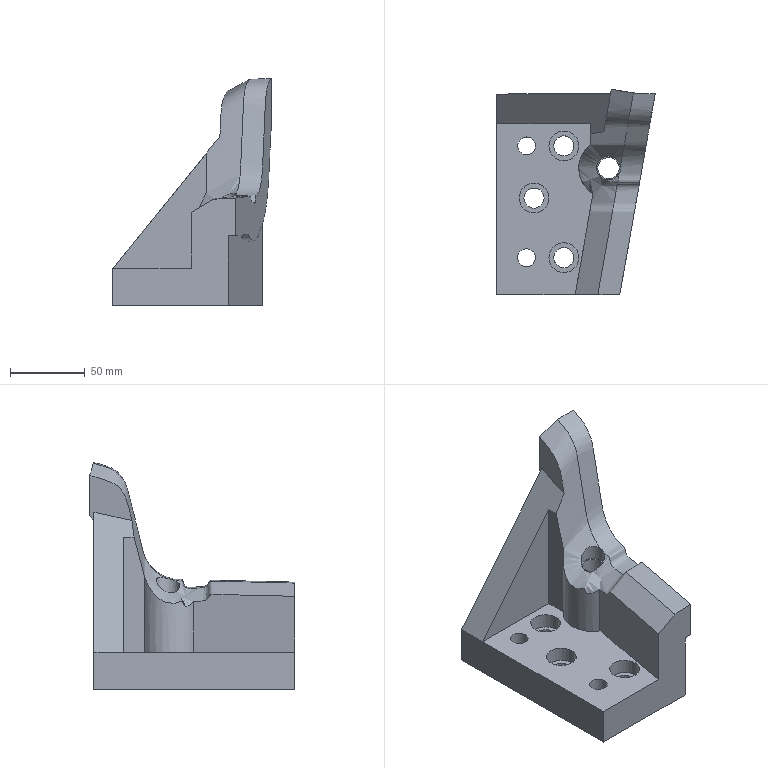Part | NX | features solid 2 | 1 solid | 33 faces | box 106.313 x 137.96 x 152.325 mm | volume 583517 mm3 | plane 13 | cylinder 11 | spline 9 | commonest cylinder face diameters 13.5 x3 20 x3 12 x2 14.376 x1 16 x1 40 x1